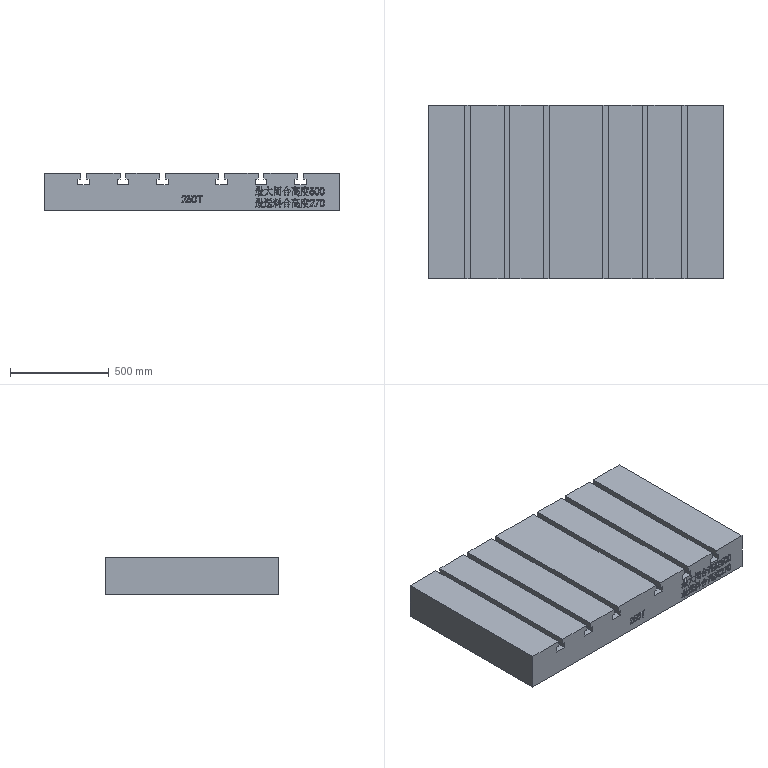Part | NX | features LIN_SOLID_COLOR 2 | 1 solid | 872 faces | box 1500 x 880 x 190 mm | volume 237781676 mm3 | plane 583 | spline 289